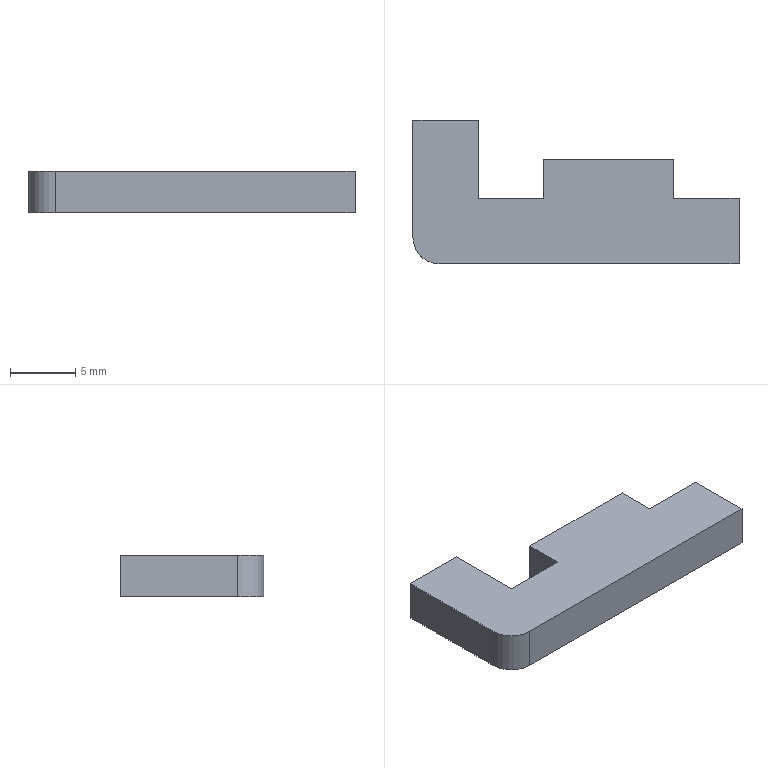Part | SolidWorks | features FlatPattern 1, SMBaseFlange 1, SheetMetal 1 | 1 solid | 13 faces | box 25 x 11 x 3.2 mm | volume 589.253 mm3 | plane 12 | cylinder 1 | commonest cylinder face diameters 4 x1
STEP:
#1=CARTESIAN_POINT('',(-99.188,173.946,0.));
#2=VERTEX_POINT('',#1);
#3=CARTESIAN_POINT('',(-104.188,173.946,0.));
#4=VERTEX_POINT('',#3);
#5=CARTESIAN_POINT('',(-104.188,173.946,0.));
#6=DIRECTION('',(-1.,0.,0.));
#7=VECTOR('',#6,1000.);
#8=LINE('',#5,#7);
#9=EDGE_CURVE('',#2,#4,#8,.T.);
#10=ORIENTED_EDGE('',*,*,#9,.F.);
#11=CARTESIAN_POINT('',(-99.188,173.946,-3.2));
#12=VERTEX_POINT('',#11);
#13=CARTESIAN_POINT('',(-99.188,173.946,-3.2));
#14=DIRECTION('',(0.,0.,1.));
#15=VECTOR('',#14,1000.);
#16=LINE('',#13,#15);
#17=EDGE_CURVE('',#12,#2,#16,.T.);
#18=ORIENTED_EDGE('',*,*,#17,.F.);
#19=CARTESIAN_POINT('',(-104.188,173.946,-3.2));
#20=VERTEX_POINT('',#19);
#21=CARTESIAN_POINT('',(-104.188,173.946,-3.2));
#22=DIRECTION('',(-1.,0.,0.));
#23=VECTOR('',#22,1000.);
#24=LINE('',#21,#23);
#25=EDGE_CURVE('',#12,#20,#24,.T.);
#26=ORIENTED_EDGE('',*,*,#25,.T.);
#27=CARTESIAN_POINT('',(-104.188,173.946,-3.2));
#28=DIRECTION('',(0.,0.,1.));
#29=VECTOR('',#28,1000.);
#30=LINE('',#27,#29);
#31=EDGE_CURVE('',#20,#4,#30,.T.);
#32=ORIENTED_EDGE('',*,*,#31,.T.);
#33=EDGE_LOOP('',(#10,#18,#26,#32));
#34=FACE_OUTER_BOUND('',#33,.T.);
#35=CARTESIAN_POINT('',(-104.188,173.946,-3.2));
#36=DIRECTION('',(0.,1.,0.));
#37=DIRECTION('',(0.,0.,1.));
#38=AXIS2_PLACEMENT_3D('',#35,#36,#37);
#39=PLANE('',#38);
#40=ADVANCED_FACE('',(#34),#39,.T.);
#41=CARTESIAN_POINT('',(-99.188,168.946,0.));
#42=VERTEX_POINT('',#41);
#43=CARTESIAN_POINT('',(-99.188,173.946,0.));
#44=DIRECTION('',(0.,1.,0.));
#45=VECTOR('',#44,1000.);
#46=LINE('',#43,#45);
#47=EDGE_CURVE('',#42,#2,#46,.T.);
#48=ORIENTED_EDGE('',*,*,#47,.F.);
#49=CARTESIAN_POINT('',(-99.188,168.946,-3.2));
#50=VERTEX_POINT('',#49);
#51=CARTESIAN_POINT('',(-99.188,168.946,-3.2));
#52=DIRECTION('',(0.,0.,1.));
#53=VECTOR('',#52,1000.);
#54=LINE('',#51,#53);
#55=EDGE_CURVE('',#50,#42,#54,.T.);
#56=ORIENTED_EDGE('',*,*,#55,.F.);
#57=CARTESIAN_POINT('',(-99.188,173.946,-3.2));
#58=DIRECTION('',(0.,1.,0.));
#59=VECTOR('',#58,1000.);
#60=LINE('',#57,#59);
#61=EDGE_CURVE('',#50,#12,#60,.T.);
#62=ORIENTED_EDGE('',*,*,#61,.T.);
#63=ORIENTED_EDGE('',*,*,#17,.T.);
#64=EDGE_LOOP('',(#48,#56,#62,#63));
#65=FACE_OUTER_BOUND('',#64,.T.);
#66=CARTESIAN_POINT('',(-99.188,173.946,-3.2));
#67=DIRECTION('',(1.,0.,0.));
#68=DIRECTION('',(0.,1.,0.));
#69=AXIS2_PLACEMENT_3D('',#66,#67,#68);
#70=PLANE('',#69);
#71=ADVANCED_FACE('',(#65),#70,.T.);
#72=CARTESIAN_POINT('',(-122.188,168.946,0.));
#73=VERTEX_POINT('',#72);
#74=CARTESIAN_POINT('',(-99.188,168.946,0.));
#75=DIRECTION('',(1.,0.,0.));
#76=VECTOR('',#75,1000.);
#77=LINE('',#74,#76);
#78=EDGE_CURVE('',#73,#42,#77,.T.);
#79=ORIENTED_EDGE('',*,*,#78,.F.);
#80=CARTESIAN_POINT('',(-122.188,168.946,-3.2));
#81=VERTEX_POINT('',#80);
#82=CARTESIAN_POINT('',(-122.188,168.946,-3.2));
#83=DIRECTION('',(0.,0.,1.));
#84=VECTOR('',#83,1000.);
#85=LINE('',#82,#84);
#86=EDGE_CURVE('',#81,#73,#85,.T.);
#87=ORIENTED_EDGE('',*,*,#86,.F.);
#88=CARTESIAN_POINT('',(-99.188,168.946,-3.2));
#89=DIRECTION('',(1.,0.,0.));
#90=VECTOR('',#89,1000.);
#91=LINE('',#88,#90);
#92=EDGE_CURVE('',#81,#50,#91,.T.);
#93=ORIENTED_EDGE('',*,*,#92,.T.);
#94=ORIENTED_EDGE('',*,*,#55,.T.);
#95=EDGE_LOOP('',(#79,#87,#93,#94));
#96=FACE_OUTER_BOUND('',#95,.T.);
#97=CARTESIAN_POINT('',(-99.188,168.946,-3.2));
#98=DIRECTION('',(0.,-1.,0.));
#99=DIRECTION('',(1.,0.,0.));
#100=AXIS2_PLACEMENT_3D('',#97,#98,#99);
#101=PLANE('',#100);
#102=ADVANCED_FACE('',(#96),#101,.T.);
#103=CARTESIAN_POINT('',(-124.188,170.946,0.));
#104=VERTEX_POINT('',#103);
#105=CARTESIAN_POINT('',(-122.188,170.946,0.));
#106=DIRECTION('',(0.,0.,1.));
#107=DIRECTION('',(-1.,0.,0.));
#108=AXIS2_PLACEMENT_3D('',#105,#106,#107);
#109=CIRCLE('',#108,2.);
#110=EDGE_CURVE('',#104,#73,#109,.T.);
#111=ORIENTED_EDGE('',*,*,#110,.F.);
#112=CARTESIAN_POINT('',(-124.188,170.946,-3.2));
#113=VERTEX_POINT('',#112);
#114=CARTESIAN_POINT('',(-124.188,170.946,-3.2));
#115=DIRECTION('',(0.,0.,1.));
#116=VECTOR('',#115,1000.);
#117=LINE('',#114,#116);
#118=EDGE_CURVE('',#113,#104,#117,.T.);
#119=ORIENTED_EDGE('',*,*,#118,.F.);
#120=CARTESIAN_POINT('',(-122.188,170.946,-3.2));
#121=DIRECTION('',(0.,0.,1.));
#122=DIRECTION('',(-1.,0.,0.));
#123=AXIS2_PLACEMENT_3D('',#120,#121,#122);
#124=CIRCLE('',#123,2.);
#125=EDGE_CURVE('',#113,#81,#124,.T.);
#126=ORIENTED_EDGE('',*,*,#125,.T.);
#127=ORIENTED_EDGE('',*,*,#86,.T.);
#128=EDGE_LOOP('',(#111,#119,#126,#127));
#129=FACE_OUTER_BOUND('',#128,.T.);
#130=CARTESIAN_POINT('',(-122.188,170.946,-3.2));
#131=DIRECTION('',(0.,0.,1.));
#132=DIRECTION('',(1.,0.,0.));
#133=AXIS2_PLACEMENT_3D('',#130,#131,#132);
#134=CYLINDRICAL_SURFACE('',#133,2.);
#135=ADVANCED_FACE('',(#129),#134,.T.);
#136=CARTESIAN_POINT('',(-124.188,179.946,0.));
#137=VERTEX_POINT('',#136);
#138=CARTESIAN_POINT('',(-124.188,170.946,0.));
#139=DIRECTION('',(0.,-1.,0.));
#140=VECTOR('',#139,1000.);
#141=LINE('',#138,#140);
#142=EDGE_CURVE('',#137,#104,#141,.T.);
#143=ORIENTED_EDGE('',*,*,#142,.F.);
#144=CARTESIAN_POINT('',(-124.188,179.946,-3.2));
#145=VERTEX_POINT('',#144);
#146=CARTESIAN_POINT('',(-124.188,179.946,-3.2));
#147=DIRECTION('',(0.,0.,1.));
#148=VECTOR('',#147,1000.);
#149=LINE('',#146,#148);
#150=EDGE_CURVE('',#145,#137,#149,.T.);
#151=ORIENTED_EDGE('',*,*,#150,.F.);
#152=CARTESIAN_POINT('',(-124.188,170.946,-3.2));
#153=DIRECTION('',(0.,-1.,0.));
#154=VECTOR('',#153,1000.);
#155=LINE('',#152,#154);
#156=EDGE_CURVE('',#145,#113,#155,.T.);
#157=ORIENTED_EDGE('',*,*,#156,.T.);
#158=ORIENTED_EDGE('',*,*,#118,.T.);
#159=EDGE_LOOP('',(#143,#151,#157,#158));
#160=FACE_OUTER_BOUND('',#159,.T.);
#161=CARTESIAN_POINT('',(-124.188,170.946,-3.2));
#162=DIRECTION('',(-1.,0.,0.));
#163=DIRECTION('',(0.,0.,1.));
#164=AXIS2_PLACEMENT_3D('',#161,#162,#163);
#165=PLANE('',#164);
#166=ADVANCED_FACE('',(#160),#165,.T.);
#167=CARTESIAN_POINT('',(-119.188,179.946,0.));
#168=VERTEX_POINT('',#167);
#169=CARTESIAN_POINT('',(-124.188,179.946,0.));
#170=DIRECTION('',(-1.,0.,0.));
#171=VECTOR('',#170,1000.);
#172=LINE('',#169,#171);
#173=EDGE_CURVE('',#168,#137,#172,.T.);
#174=ORIENTED_EDGE('',*,*,#173,.F.);
#175=CARTESIAN_POINT('',(-119.188,179.946,-3.2));
#176=VERTEX_POINT('',#175);
#177=CARTESIAN_POINT('',(-119.188,179.946,-3.2));
#178=DIRECTION('',(0.,0.,1.));
#179=VECTOR('',#178,1000.);
#180=LINE('',#177,#179);
#181=EDGE_CURVE('',#176,#168,#180,.T.);
#182=ORIENTED_EDGE('',*,*,#181,.F.);
#183=CARTESIAN_POINT('',(-124.188,179.946,-3.2));
#184=DIRECTION('',(-1.,0.,0.));
#185=VECTOR('',#184,1000.);
#186=LINE('',#183,#185);
#187=EDGE_CURVE('',#176,#145,#186,.T.);
#188=ORIENTED_EDGE('',*,*,#187,.T.);
#189=ORIENTED_EDGE('',*,*,#150,.T.);
#190=EDGE_LOOP('',(#174,#182,#188,#189));
#191=FACE_OUTER_BOUND('',#190,.T.);
#192=CARTESIAN_POINT('',(-124.188,179.946,-3.2));
#193=DIRECTION('',(0.,1.,0.));
#194=DIRECTION('',(0.,0.,1.));
#195=AXIS2_PLACEMENT_3D('',#192,#193,#194);
#196=PLANE('',#195);
#197=ADVANCED_FACE('',(#191),#196,.T.);
#198=CARTESIAN_POINT('',(-119.188,173.946,0.));
#199=VERTEX_POINT('',#198);
#200=CARTESIAN_POINT('',(-119.188,179.946,0.));
#201=DIRECTION('',(0.,1.,0.));
#202=VECTOR('',#201,1000.);
#203=LINE('',#200,#202);
#204=EDGE_CURVE('',#199,#168,#203,.T.);
#205=ORIENTED_EDGE('',*,*,#204,.F.);
#206=CARTESIAN_POINT('',(-119.188,173.946,-3.2));
#207=VERTEX_POINT('',#206);
#208=CARTESIAN_POINT('',(-119.188,173.946,-3.2));
#209=DIRECTION('',(0.,0.,1.));
#210=VECTOR('',#209,1000.);
#211=LINE('',#208,#210);
#212=EDGE_CURVE('',#207,#199,#211,.T.);
#213=ORIENTED_EDGE('',*,*,#212,.F.);
#214=CARTESIAN_POINT('',(-119.188,179.946,-3.2));
#215=DIRECTION('',(0.,1.,0.));
#216=VECTOR('',#215,1000.);
#217=LINE('',#214,#216);
#218=EDGE_CURVE('',#207,#176,#217,.T.);
#219=ORIENTED_EDGE('',*,*,#218,.T.);
#220=ORIENTED_EDGE('',*,*,#181,.T.);
#221=EDGE_LOOP('',(#205,#213,#219,#220));
#222=FACE_OUTER_BOUND('',#221,.T.);
#223=CARTESIAN_POINT('',(-119.188,179.946,-3.2));
#224=DIRECTION('',(1.,0.,0.));
#225=DIRECTION('',(0.,0.,-1.));
#226=AXIS2_PLACEMENT_3D('',#223,#224,#225);
#227=PLANE('',#226);
#228=ADVANCED_FACE('',(#222),#227,.T.);
#229=CARTESIAN_POINT('',(-114.188,173.946,0.));
#230=VERTEX_POINT('',#229);
#231=CARTESIAN_POINT('',(-119.188,173.946,0.));
#232=DIRECTION('',(-1.,0.,0.));
#233=VECTOR('',#232,1000.);
#234=LINE('',#231,#233);
#235=EDGE_CURVE('',#230,#199,#234,.T.);
#236=ORIENTED_EDGE('',*,*,#235,.F.);
#237=CARTESIAN_POINT('',(-114.188,173.946,-3.2));
#238=VERTEX_POINT('',#237);
#239=CARTESIAN_POINT('',(-114.188,173.946,-3.2));
#240=DIRECTION('',(0.,0.,1.));
#241=VECTOR('',#240,1000.);
#242=LINE('',#239,#241);
#243=EDGE_CURVE('',#238,#230,#242,.T.);
#244=ORIENTED_EDGE('',*,*,#243,.F.);
#245=CARTESIAN_POINT('',(-119.188,173.946,-3.2));
#246=DIRECTION('',(-1.,0.,0.));
#247=VECTOR('',#246,1000.);
#248=LINE('',#245,#247);
#249=EDGE_CURVE('',#238,#207,#248,.T.);
#250=ORIENTED_EDGE('',*,*,#249,.T.);
#251=ORIENTED_EDGE('',*,*,#212,.T.);
#252=EDGE_LOOP('',(#236,#244,#250,#251));
#253=FACE_OUTER_BOUND('',#252,.T.);
#254=CARTESIAN_POINT('',(-119.188,173.946,-3.2));
#255=DIRECTION('',(0.,1.,0.));
#256=DIRECTION('',(0.,0.,1.));
#257=AXIS2_PLACEMENT_3D('',#254,#255,#256);
#258=PLANE('',#257);
#259=ADVANCED_FACE('',(#253),#258,.T.);
#260=CARTESIAN_POINT('',(-114.188,176.946,0.));
#261=VERTEX_POINT('',#260);
#262=CARTESIAN_POINT('',(-114.188,173.946,0.));
#263=DIRECTION('',(0.,-1.,0.));
#264=VECTOR('',#263,1000.);
#265=LINE('',#262,#264);
#266=EDGE_CURVE('',#261,#230,#265,.T.);
#267=ORIENTED_EDGE('',*,*,#266,.F.);
#268=CARTESIAN_POINT('',(-114.188,176.946,-3.2));
#269=VERTEX_POINT('',#268);
#270=CARTESIAN_POINT('',(-114.188,176.946,-3.2));
#271=DIRECTION('',(0.,0.,1.));
#272=VECTOR('',#271,1000.);
#273=LINE('',#270,#272);
#274=EDGE_CURVE('',#269,#261,#273,.T.);
#275=ORIENTED_EDGE('',*,*,#274,.F.);
#276=CARTESIAN_POINT('',(-114.188,173.946,-3.2));
#277=DIRECTION('',(0.,-1.,0.));
#278=VECTOR('',#277,1000.);
#279=LINE('',#276,#278);
#280=EDGE_CURVE('',#269,#238,#279,.T.);
#281=ORIENTED_EDGE('',*,*,#280,.T.);
#282=ORIENTED_EDGE('',*,*,#243,.T.);
#283=EDGE_LOOP('',(#267,#275,#281,#282));
#284=FACE_OUTER_BOUND('',#283,.T.);
#285=CARTESIAN_POINT('',(-114.188,173.946,-3.2));
#286=DIRECTION('',(-1.,0.,0.));
#287=DIRECTION('',(0.,0.,1.));
#288=AXIS2_PLACEMENT_3D('',#285,#286,#287);
#289=PLANE('',#288);
#290=ADVANCED_FACE('',(#284),#289,.T.);
#291=CARTESIAN_POINT('',(-104.188,176.946,0.));
#292=VERTEX_POINT('',#291);
#293=CARTESIAN_POINT('',(-114.188,176.946,0.));
#294=DIRECTION('',(-1.,0.,0.));
#295=VECTOR('',#294,1000.);
#296=LINE('',#293,#295);
#297=EDGE_CURVE('',#292,#261,#296,.T.);
#298=ORIENTED_EDGE('',*,*,#297,.F.);
#299=CARTESIAN_POINT('',(-104.188,176.946,-3.2));
#300=VERTEX_POINT('',#299);
#301=CARTESIAN_POINT('',(-104.188,176.946,-3.2));
#302=DIRECTION('',(0.,0.,1.));
#303=VECTOR('',#302,1000.);
#304=LINE('',#301,#303);
#305=EDGE_CURVE('',#300,#292,#304,.T.);
#306=ORIENTED_EDGE('',*,*,#305,.F.);
#307=CARTESIAN_POINT('',(-114.188,176.946,-3.2));
#308=DIRECTION('',(-1.,0.,0.));
#309=VECTOR('',#308,1000.);
#310=LINE('',#307,#309);
#311=EDGE_CURVE('',#300,#269,#310,.T.);
#312=ORIENTED_EDGE('',*,*,#311,.T.);
#313=ORIENTED_EDGE('',*,*,#274,.T.);
#314=EDGE_LOOP('',(#298,#306,#312,#313));
#315=FACE_OUTER_BOUND('',#314,.T.);
#316=CARTESIAN_POINT('',(-114.188,176.946,-3.2));
#317=DIRECTION('',(0.,1.,0.));
#318=DIRECTION('',(0.,0.,1.));
#319=AXIS2_PLACEMENT_3D('',#316,#317,#318);
#320=PLANE('',#319);
#321=ADVANCED_FACE('',(#315),#320,.T.);
#322=CARTESIAN_POINT('',(-104.188,176.946,0.));
#323=DIRECTION('',(0.,1.,0.));
#324=VECTOR('',#323,1000.);
#325=LINE('',#322,#324);
#326=EDGE_CURVE('',#4,#292,#325,.T.);
#327=ORIENTED_EDGE('',*,*,#326,.F.);
#328=ORIENTED_EDGE('',*,*,#31,.F.);
#329=CARTESIAN_POINT('',(-104.188,176.946,-3.2));
#330=DIRECTION('',(0.,1.,0.));
#331=VECTOR('',#330,1000.);
#332=LINE('',#329,#331);
#333=EDGE_CURVE('',#20,#300,#332,.T.);
#334=ORIENTED_EDGE('',*,*,#333,.T.);
#335=ORIENTED_EDGE('',*,*,#305,.T.);
#336=EDGE_LOOP('',(#327,#328,#334,#335));
#337=FACE_OUTER_BOUND('',#336,.T.);
#338=CARTESIAN_POINT('',(-104.188,176.946,-3.2));
#339=DIRECTION('',(1.,0.,0.));
#340=DIRECTION('',(0.,0.,-1.));
#341=AXIS2_PLACEMENT_3D('',#338,#339,#340);
#342=PLANE('',#341);
#343=ADVANCED_FACE('',(#337),#342,.T.);
#344=ORIENTED_EDGE('',*,*,#25,.F.);
#345=ORIENTED_EDGE('',*,*,#61,.F.);
#346=ORIENTED_EDGE('',*,*,#92,.F.);
#347=ORIENTED_EDGE('',*,*,#125,.F.);
#348=ORIENTED_EDGE('',*,*,#156,.F.);
#349=ORIENTED_EDGE('',*,*,#187,.F.);
#350=ORIENTED_EDGE('',*,*,#218,.F.);
#351=ORIENTED_EDGE('',*,*,#249,.F.);
#352=ORIENTED_EDGE('',*,*,#280,.F.);
#353=ORIENTED_EDGE('',*,*,#311,.F.);
#354=ORIENTED_EDGE('',*,*,#333,.F.);
#355=EDGE_LOOP('',(#344,#345,#346,#347,#348,#349,#350,#351,#352,#353,#354));
#356=FACE_OUTER_BOUND('',#355,.T.);
#357=CARTESIAN_POINT('',(-122.188,170.946,-3.2));
#358=DIRECTION('',(0.,0.,-1.));
#359=DIRECTION('',(-1.,0.,0.));
#360=AXIS2_PLACEMENT_3D('',#357,#358,#359);
#361=PLANE('',#360);
#362=ADVANCED_FACE('',(#356),#361,.T.);
#363=ORIENTED_EDGE('',*,*,#9,.T.);
#364=ORIENTED_EDGE('',*,*,#326,.T.);
#365=ORIENTED_EDGE('',*,*,#297,.T.);
#366=ORIENTED_EDGE('',*,*,#266,.T.);
#367=ORIENTED_EDGE('',*,*,#235,.T.);
#368=ORIENTED_EDGE('',*,*,#204,.T.);
#369=ORIENTED_EDGE('',*,*,#173,.T.);
#370=ORIENTED_EDGE('',*,*,#142,.T.);
#371=ORIENTED_EDGE('',*,*,#110,.T.);
#372=ORIENTED_EDGE('',*,*,#78,.T.);
#373=ORIENTED_EDGE('',*,*,#47,.T.);
#374=EDGE_LOOP('',(#363,#364,#365,#366,#367,#368,#369,#370,#371,#372,#373));
#375=FACE_OUTER_BOUND('',#374,.T.);
#376=CARTESIAN_POINT('',(-122.188,170.946,0.));
#377=DIRECTION('',(0.,0.,-1.));
#378=DIRECTION('',(-1.,0.,0.));
#379=AXIS2_PLACEMENT_3D('',#376,#377,#378);
#380=PLANE('',#379);
#381=ADVANCED_FACE('',(#375),#380,.F.);
#382=CLOSED_SHELL('',(#40,#71,#102,#135,#166,#197,#228,#259,#290,#321,#343,#362,#381));
#383=MANIFOLD_SOLID_BREP('',#382);
#384=CARTESIAN_POINT('',(0.,0.,0.));
#385=DIRECTION('',(0.,0.,1.));
#386=DIRECTION('',(1.,0.,0.));
#387=AXIS2_PLACEMENT_3D('',#384,#385,#386);
#388=(LENGTH_UNIT()NAMED_UNIT(*)SI_UNIT(.MILLI.,.METRE.));
#389=UNCERTAINTY_MEASURE_WITH_UNIT(LENGTH_MEASURE(0.00001),#388,'','');
#390=(NAMED_UNIT(*)PLANE_ANGLE_UNIT()SI_UNIT($,.RADIAN.));
#391=(NAMED_UNIT(*)SI_UNIT($,.STERADIAN.)SOLID_ANGLE_UNIT());
#392=(GEOMETRIC_REPRESENTATION_CONTEXT(3)GLOBAL_UNCERTAINTY_ASSIGNED_CONTEXT((#389))GLOBAL_UNIT_ASSIGNED_CONTEXT((#388,#390,#391))REPRESENTATION_CONTEXT('',''));
#393=ADVANCED_BREP_SHAPE_REPRESENTATION('',(#383,#387),#392);